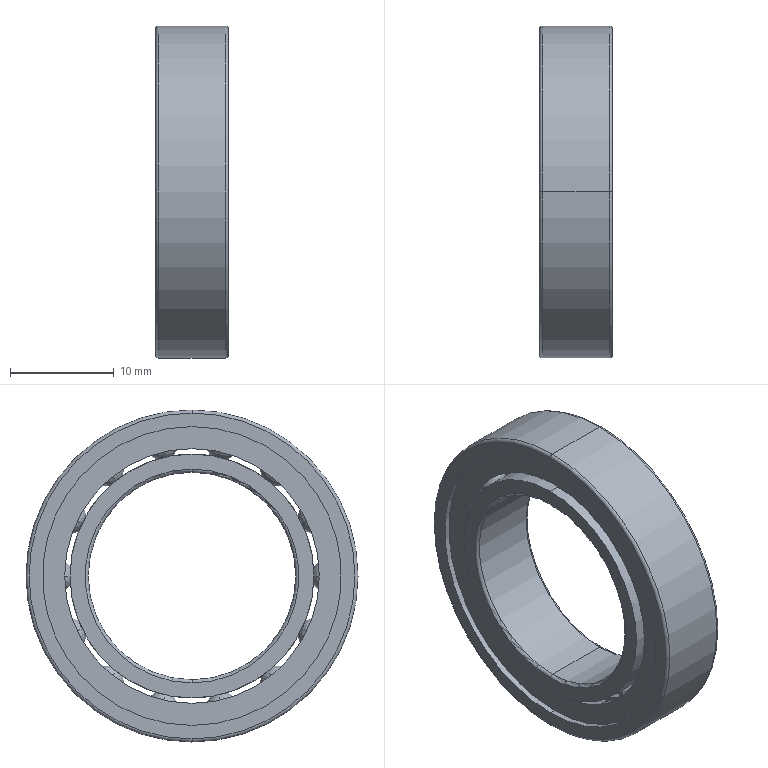Part | STEP file | GB/T 276 61804_61804-2Z | 1 solid | 225 faces | box 7 x 32 x 32 mm | volume 2319 mm3 | sphere 112 | torus 53 | plane 36 | cylinder 24 | commonest cylinder face diameters 28.8 x8 23.5 x4 24.548 x4 20 x2 25.277 x2 27.023 x2